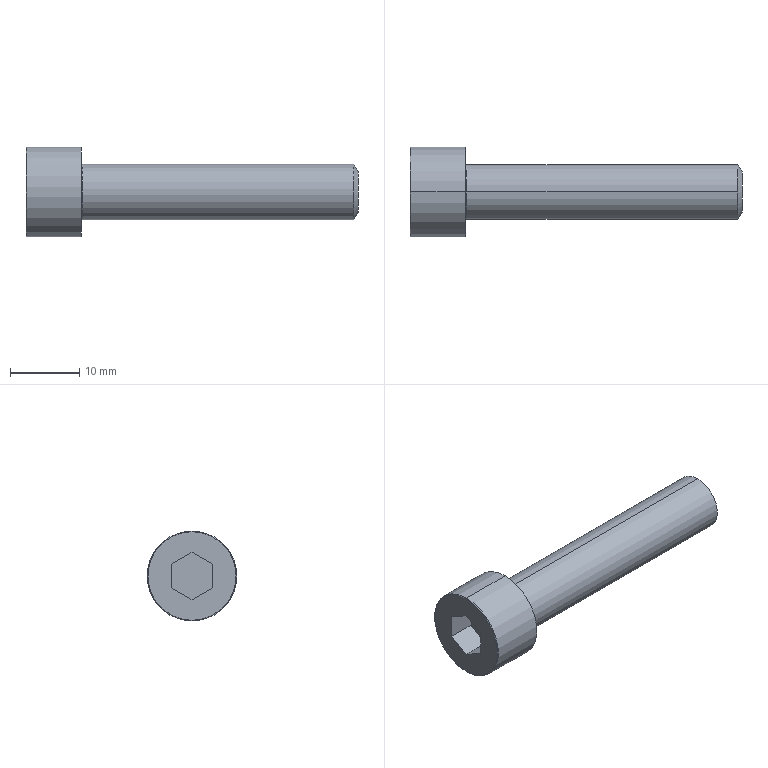Part | SolidWorks | features BlendCut 1, Cut 1, Fillet 1, LPattern 1, RevCut 1, Revolution 1 | 1 solid | 20 faces | box 48 x 13 x 13 mm | volume 2943 mm3 | plane 10 | torus 4 | cylinder 4 | cone 2 | commonest cylinder face diameters 8 x2 13 x2
STEP:
#1=CARTESIAN_POINT('',(0.,0.,6.4));
#2=VERTEX_POINT('',#1);
#3=CARTESIAN_POINT('',(0.,0.,-6.4));
#4=VERTEX_POINT('',#3);
#5=CARTESIAN_POINT('',(0.,0.,0.));
#6=DIRECTION('',(-1.,0.,0.));
#7=DIRECTION('',(0.,0.,-1.));
#8=AXIS2_PLACEMENT_3D('',#5,#6,#7);
#9=CIRCLE('',#8,6.4);
#10=EDGE_CURVE('',#2,#4,#9,.T.);
#11=ORIENTED_EDGE('',*,*,#10,.F.);
#12=CARTESIAN_POINT('',(0.1,0.,6.5));
#13=VERTEX_POINT('',#12);
#14=CARTESIAN_POINT('',(0.1,0.,6.4));
#15=DIRECTION('',(0.,1.,0.));
#16=DIRECTION('',(0.,0.,1.));
#17=AXIS2_PLACEMENT_3D('',#14,#15,#16);
#18=CIRCLE('',#17,0.1);
#19=EDGE_CURVE('',#2,#13,#18,.T.);
#20=ORIENTED_EDGE('',*,*,#19,.T.);
#21=CARTESIAN_POINT('',(0.1,0.,-6.5));
#22=VERTEX_POINT('',#21);
#23=CARTESIAN_POINT('',(0.1,0.,0.));
#24=DIRECTION('',(1.,0.,0.));
#25=DIRECTION('',(0.,0.,-1.));
#26=AXIS2_PLACEMENT_3D('',#23,#24,#25);
#27=CIRCLE('',#26,6.5);
#28=EDGE_CURVE('',#22,#13,#27,.T.);
#29=ORIENTED_EDGE('',*,*,#28,.F.);
#30=CARTESIAN_POINT('',(0.1,0.,-6.4));
#31=DIRECTION('',(0.,-1.,0.));
#32=DIRECTION('',(0.,0.,-1.));
#33=AXIS2_PLACEMENT_3D('',#30,#31,#32);
#34=CIRCLE('',#33,0.1);
#35=EDGE_CURVE('',#4,#22,#34,.T.);
#36=ORIENTED_EDGE('',*,*,#35,.F.);
#37=EDGE_LOOP('',(#11,#20,#29,#36));
#38=FACE_OUTER_BOUND('',#37,.T.);
#39=CARTESIAN_POINT('',(0.1,0.,0.));
#40=DIRECTION('',(1.,0.,0.));
#41=DIRECTION('',(0.,0.,-1.));
#42=AXIS2_PLACEMENT_3D('',#39,#40,#41);
#43=TOROIDAL_SURFACE('',#42,6.4,0.1);
#44=ADVANCED_FACE('',(#38),#43,.T.);
#45=CARTESIAN_POINT('',(48.,0.,2.917));
#46=VERTEX_POINT('',#45);
#47=CARTESIAN_POINT('',(48.,0.,-2.917));
#48=VERTEX_POINT('',#47);
#49=CARTESIAN_POINT('',(48.,0.,0.));
#50=DIRECTION('',(-1.,0.,0.));
#51=DIRECTION('',(0.,0.,1.));
#52=AXIS2_PLACEMENT_3D('',#49,#50,#51);
#53=CIRCLE('',#52,2.917);
#54=EDGE_CURVE('',#46,#48,#53,.T.);
#55=ORIENTED_EDGE('',*,*,#54,.T.);
#56=CARTESIAN_POINT('',(47.375,0.,-4.));
#57=VERTEX_POINT('',#56);
#58=CARTESIAN_POINT('',(47.375,0.,-4.));
#59=DIRECTION('',(-0.5,0.,-0.866));
#60=VECTOR('',#59,1000.);
#61=LINE('',#58,#60);
#62=EDGE_CURVE('',#48,#57,#61,.T.);
#63=ORIENTED_EDGE('',*,*,#62,.T.);
#64=CARTESIAN_POINT('',(47.375,0.,4.));
#65=VERTEX_POINT('',#64);
#66=CARTESIAN_POINT('',(47.375,0.,0.));
#67=DIRECTION('',(-1.,0.,0.));
#68=DIRECTION('',(0.,0.,1.));
#69=AXIS2_PLACEMENT_3D('',#66,#67,#68);
#70=CIRCLE('',#69,4.);
#71=EDGE_CURVE('',#65,#57,#70,.T.);
#72=ORIENTED_EDGE('',*,*,#71,.F.);
#73=CARTESIAN_POINT('',(47.375,0.,4.));
#74=DIRECTION('',(-0.5,0.,0.866));
#75=VECTOR('',#74,1000.);
#76=LINE('',#73,#75);
#77=EDGE_CURVE('',#46,#65,#76,.T.);
#78=ORIENTED_EDGE('',*,*,#77,.F.);
#79=EDGE_LOOP('',(#55,#63,#72,#78));
#80=FACE_OUTER_BOUND('',#79,.T.);
#81=CARTESIAN_POINT('',(47.375,0.,0.));
#82=DIRECTION('',(-1.,0.,0.));
#83=DIRECTION('',(0.,0.,1.));
#84=AXIS2_PLACEMENT_3D('',#81,#82,#83);
#85=CONICAL_SURFACE('',#84,4.,1.047);
#86=ADVANCED_FACE('',(#80),#85,.T.);
#87=CARTESIAN_POINT('',(8.,0.,-4.2));
#88=VERTEX_POINT('',#87);
#89=CARTESIAN_POINT('',(8.,0.,4.2));
#90=VERTEX_POINT('',#89);
#91=CARTESIAN_POINT('',(8.,0.,0.));
#92=DIRECTION('',(-1.,0.,0.));
#93=DIRECTION('',(0.,0.,1.));
#94=AXIS2_PLACEMENT_3D('',#91,#92,#93);
#95=CIRCLE('',#94,4.2);
#96=EDGE_CURVE('',#88,#90,#95,.T.);
#97=ORIENTED_EDGE('',*,*,#96,.F.);
#98=CARTESIAN_POINT('',(8.2,0.,-4.));
#99=VERTEX_POINT('',#98);
#100=CARTESIAN_POINT('',(8.2,0.,-4.2));
#101=DIRECTION('',(0.,1.,0.));
#102=DIRECTION('',(0.,0.,1.));
#103=AXIS2_PLACEMENT_3D('',#100,#101,#102);
#104=CIRCLE('',#103,0.2);
#105=EDGE_CURVE('',#88,#99,#104,.T.);
#106=ORIENTED_EDGE('',*,*,#105,.T.);
#107=CARTESIAN_POINT('',(8.2,0.,4.));
#108=VERTEX_POINT('',#107);
#109=CARTESIAN_POINT('',(8.2,0.,0.));
#110=DIRECTION('',(-1.,0.,0.));
#111=DIRECTION('',(0.,0.,1.));
#112=AXIS2_PLACEMENT_3D('',#109,#110,#111);
#113=CIRCLE('',#112,4.);
#114=EDGE_CURVE('',#99,#108,#113,.T.);
#115=ORIENTED_EDGE('',*,*,#114,.T.);
#116=CARTESIAN_POINT('',(8.2,0.,4.2));
#117=DIRECTION('',(0.,-1.,0.));
#118=DIRECTION('',(0.,0.,-1.));
#119=AXIS2_PLACEMENT_3D('',#116,#117,#118);
#120=CIRCLE('',#119,0.2);
#121=EDGE_CURVE('',#90,#108,#120,.T.);
#122=ORIENTED_EDGE('',*,*,#121,.F.);
#123=EDGE_LOOP('',(#97,#106,#115,#122));
#124=FACE_OUTER_BOUND('',#123,.T.);
#125=CARTESIAN_POINT('',(8.2,0.,0.));
#126=DIRECTION('',(-1.,0.,0.));
#127=DIRECTION('',(0.,0.,1.));
#128=AXIS2_PLACEMENT_3D('',#125,#126,#127);
#129=TOROIDAL_SURFACE('',#128,4.2,0.2);
#130=ADVANCED_FACE('',(#124),#129,.F.);
#131=CARTESIAN_POINT('',(8.,0.,6.5));
#132=VERTEX_POINT('',#131);
#133=CARTESIAN_POINT('',(8.,0.,-6.5));
#134=VERTEX_POINT('',#133);
#135=CARTESIAN_POINT('',(8.,0.,0.));
#136=DIRECTION('',(-1.,0.,0.));
#137=DIRECTION('',(0.,0.,1.));
#138=AXIS2_PLACEMENT_3D('',#135,#136,#137);
#139=CIRCLE('',#138,6.5);
#140=EDGE_CURVE('',#132,#134,#139,.T.);
#141=ORIENTED_EDGE('',*,*,#140,.T.);
#142=CARTESIAN_POINT('',(0.,0.,-6.5));
#143=DIRECTION('',(-1.,0.,0.));
#144=VECTOR('',#143,1000.);
#145=LINE('',#142,#144);
#146=EDGE_CURVE('',#134,#22,#145,.T.);
#147=ORIENTED_EDGE('',*,*,#146,.T.);
#148=ORIENTED_EDGE('',*,*,#28,.T.);
#149=CARTESIAN_POINT('',(0.,0.,6.5));
#150=DIRECTION('',(-1.,0.,0.));
#151=VECTOR('',#150,1000.);
#152=LINE('',#149,#151);
#153=EDGE_CURVE('',#132,#13,#152,.T.);
#154=ORIENTED_EDGE('',*,*,#153,.F.);
#155=EDGE_LOOP('',(#141,#147,#148,#154));
#156=FACE_OUTER_BOUND('',#155,.T.);
#157=CARTESIAN_POINT('',(0.,0.,0.));
#158=DIRECTION('',(-1.,0.,0.));
#159=DIRECTION('',(0.,0.,1.));
#160=AXIS2_PLACEMENT_3D('',#157,#158,#159);
#161=CYLINDRICAL_SURFACE('',#160,6.5);
#162=ADVANCED_FACE('',(#156),#161,.T.);
#163=ORIENTED_EDGE('',*,*,#71,.T.);
#164=CARTESIAN_POINT('',(0.,0.,-4.));
#165=DIRECTION('',(-1.,0.,0.));
#166=VECTOR('',#165,1000.);
#167=LINE('',#164,#166);
#168=EDGE_CURVE('',#57,#99,#167,.T.);
#169=ORIENTED_EDGE('',*,*,#168,.T.);
#170=CARTESIAN_POINT('',(8.2,0.,0.));
#171=DIRECTION('',(-1.,0.,0.));
#172=DIRECTION('',(0.,0.,1.));
#173=AXIS2_PLACEMENT_3D('',#170,#171,#172);
#174=CIRCLE('',#173,4.);
#175=EDGE_CURVE('',#108,#99,#174,.T.);
#176=ORIENTED_EDGE('',*,*,#175,.F.);
#177=CARTESIAN_POINT('',(0.,0.,4.));
#178=DIRECTION('',(-1.,0.,0.));
#179=VECTOR('',#178,1000.);
#180=LINE('',#177,#179);
#181=EDGE_CURVE('',#65,#108,#180,.T.);
#182=ORIENTED_EDGE('',*,*,#181,.F.);
#183=EDGE_LOOP('',(#163,#169,#176,#182));
#184=FACE_OUTER_BOUND('',#183,.T.);
#185=CARTESIAN_POINT('',(0.,0.,0.));
#186=DIRECTION('',(-1.,0.,0.));
#187=DIRECTION('',(0.,0.,1.));
#188=AXIS2_PLACEMENT_3D('',#185,#186,#187);
#189=CYLINDRICAL_SURFACE('',#188,4.);
#190=ADVANCED_FACE('',(#184),#189,.T.);
#191=ORIENTED_EDGE('',*,*,#168,.F.);
#192=CARTESIAN_POINT('',(47.375,0.,0.));
#193=DIRECTION('',(-1.,0.,0.));
#194=DIRECTION('',(0.,0.,1.));
#195=AXIS2_PLACEMENT_3D('',#192,#193,#194);
#196=CIRCLE('',#195,4.);
#197=EDGE_CURVE('',#57,#65,#196,.T.);
#198=ORIENTED_EDGE('',*,*,#197,.T.);
#199=ORIENTED_EDGE('',*,*,#181,.T.);
#200=ORIENTED_EDGE('',*,*,#114,.F.);
#201=EDGE_LOOP('',(#191,#198,#199,#200));
#202=FACE_OUTER_BOUND('',#201,.T.);
#203=CARTESIAN_POINT('',(0.,0.,0.));
#204=DIRECTION('',(-1.,0.,0.));
#205=DIRECTION('',(0.,0.,1.));
#206=AXIS2_PLACEMENT_3D('',#203,#204,#205);
#207=CYLINDRICAL_SURFACE('',#206,4.);
#208=ADVANCED_FACE('',(#202),#207,.T.);
#209=CARTESIAN_POINT('',(0.,0.,0.));
#210=DIRECTION('',(-1.,0.,0.));
#211=DIRECTION('',(0.,0.,-1.));
#212=AXIS2_PLACEMENT_3D('',#209,#210,#211);
#213=CIRCLE('',#212,6.4);
#214=EDGE_CURVE('',#4,#2,#213,.T.);
#215=ORIENTED_EDGE('',*,*,#214,.T.);
#216=ORIENTED_EDGE('',*,*,#10,.T.);
#217=EDGE_LOOP('',(#215,#216));
#218=FACE_OUTER_BOUND('',#217,.T.);
#219=CARTESIAN_POINT('',(0.,0.,3.43));
#220=VERTEX_POINT('',#219);
#221=CARTESIAN_POINT('',(0.,2.97,1.715));
#222=VERTEX_POINT('',#221);
#223=CARTESIAN_POINT('',(0.,0.,3.43));
#224=DIRECTION('',(0.,0.866,-0.5));
#225=VECTOR('',#224,1000.);
#226=LINE('',#223,#225);
#227=EDGE_CURVE('',#220,#222,#226,.T.);
#228=ORIENTED_EDGE('',*,*,#227,.F.);
#229=CARTESIAN_POINT('',(0.,-2.97,1.715));
#230=VERTEX_POINT('',#229);
#231=CARTESIAN_POINT('',(0.,-2.97,1.715));
#232=DIRECTION('',(0.,0.866,0.5));
#233=VECTOR('',#232,1000.);
#234=LINE('',#231,#233);
#235=EDGE_CURVE('',#230,#220,#234,.T.);
#236=ORIENTED_EDGE('',*,*,#235,.F.);
#237=CARTESIAN_POINT('',(0.,-2.97,-1.715));
#238=VERTEX_POINT('',#237);
#239=CARTESIAN_POINT('',(0.,-2.97,-1.715));
#240=DIRECTION('',(0.,0.,1.));
#241=VECTOR('',#240,1000.);
#242=LINE('',#239,#241);
#243=EDGE_CURVE('',#238,#230,#242,.T.);
#244=ORIENTED_EDGE('',*,*,#243,.F.);
#245=CARTESIAN_POINT('',(0.,0.,-3.43));
#246=VERTEX_POINT('',#245);
#247=CARTESIAN_POINT('',(0.,0.,-3.43));
#248=DIRECTION('',(0.,-0.866,0.5));
#249=VECTOR('',#248,1000.);
#250=LINE('',#247,#249);
#251=EDGE_CURVE('',#246,#238,#250,.T.);
#252=ORIENTED_EDGE('',*,*,#251,.F.);
#253=CARTESIAN_POINT('',(0.,2.97,-1.715));
#254=VERTEX_POINT('',#253);
#255=CARTESIAN_POINT('',(0.,2.97,-1.715));
#256=DIRECTION('',(0.,-0.866,-0.5));
#257=VECTOR('',#256,1000.);
#258=LINE('',#255,#257);
#259=EDGE_CURVE('',#254,#246,#258,.T.);
#260=ORIENTED_EDGE('',*,*,#259,.F.);
#261=CARTESIAN_POINT('',(0.,2.97,1.715));
#262=DIRECTION('',(0.,0.,-1.));
#263=VECTOR('',#262,1000.);
#264=LINE('',#261,#263);
#265=EDGE_CURVE('',#222,#254,#264,.T.);
#266=ORIENTED_EDGE('',*,*,#265,.F.);
#267=EDGE_LOOP('',(#228,#236,#244,#252,#260,#266));
#268=FACE_BOUND('',#267,.T.);
#269=CARTESIAN_POINT('',(0.,0.,0.));
#270=DIRECTION('',(1.,0.,0.));
#271=DIRECTION('',(0.,0.,-1.));
#272=AXIS2_PLACEMENT_3D('',#269,#270,#271);
#273=PLANE('',#272);
#274=ADVANCED_FACE('',(#218,#268),#273,.F.);
#275=ORIENTED_EDGE('',*,*,#146,.F.);
#276=CARTESIAN_POINT('',(8.,0.,0.));
#277=DIRECTION('',(-1.,0.,0.));
#278=DIRECTION('',(0.,0.,1.));
#279=AXIS2_PLACEMENT_3D('',#276,#277,#278);
#280=CIRCLE('',#279,6.5);
#281=EDGE_CURVE('',#134,#132,#280,.T.);
#282=ORIENTED_EDGE('',*,*,#281,.T.);
#283=ORIENTED_EDGE('',*,*,#153,.T.);
#284=CARTESIAN_POINT('',(0.1,0.,0.));
#285=DIRECTION('',(1.,0.,0.));
#286=DIRECTION('',(0.,0.,-1.));
#287=AXIS2_PLACEMENT_3D('',#284,#285,#286);
#288=CIRCLE('',#287,6.5);
#289=EDGE_CURVE('',#13,#22,#288,.T.);
#290=ORIENTED_EDGE('',*,*,#289,.T.);
#291=EDGE_LOOP('',(#275,#282,#283,#290));
#292=FACE_OUTER_BOUND('',#291,.T.);
#293=CARTESIAN_POINT('',(0.,0.,0.));
#294=DIRECTION('',(-1.,0.,0.));
#295=DIRECTION('',(0.,0.,1.));
#296=AXIS2_PLACEMENT_3D('',#293,#294,#295);
#297=CYLINDRICAL_SURFACE('',#296,6.5);
#298=ADVANCED_FACE('',(#292),#297,.T.);
#299=ORIENTED_EDGE('',*,*,#140,.F.);
#300=ORIENTED_EDGE('',*,*,#281,.F.);
#301=EDGE_LOOP('',(#299,#300));
#302=FACE_OUTER_BOUND('',#301,.T.);
#303=CARTESIAN_POINT('',(8.,0.,0.));
#304=DIRECTION('',(-1.,0.,0.));
#305=DIRECTION('',(0.,0.,1.));
#306=AXIS2_PLACEMENT_3D('',#303,#304,#305);
#307=CIRCLE('',#306,4.2);
#308=EDGE_CURVE('',#90,#88,#307,.T.);
#309=ORIENTED_EDGE('',*,*,#308,.T.);
#310=ORIENTED_EDGE('',*,*,#96,.T.);
#311=EDGE_LOOP('',(#309,#310));
#312=FACE_BOUND('',#311,.T.);
#313=CARTESIAN_POINT('',(8.,6.5,0.));
#314=DIRECTION('',(-1.,0.,0.));
#315=DIRECTION('',(0.,0.,1.));
#316=AXIS2_PLACEMENT_3D('',#313,#314,#315);
#317=PLANE('',#316);
#318=ADVANCED_FACE('',(#302,#312),#317,.F.);
#319=ORIENTED_EDGE('',*,*,#105,.F.);
#320=ORIENTED_EDGE('',*,*,#308,.F.);
#321=ORIENTED_EDGE('',*,*,#121,.T.);
#322=ORIENTED_EDGE('',*,*,#175,.T.);
#323=EDGE_LOOP('',(#319,#320,#321,#322));
#324=FACE_OUTER_BOUND('',#323,.T.);
#325=CARTESIAN_POINT('',(8.2,0.,0.));
#326=DIRECTION('',(-1.,0.,0.));
#327=DIRECTION('',(0.,0.,1.));
#328=AXIS2_PLACEMENT_3D('',#325,#326,#327);
#329=TOROIDAL_SURFACE('',#328,4.2,0.2);
#330=ADVANCED_FACE('',(#324),#329,.F.);
#331=ORIENTED_EDGE('',*,*,#235,.T.);
#332=CARTESIAN_POINT('',(4.,0.,3.43));
#333=VERTEX_POINT('',#332);
#334=CARTESIAN_POINT('',(4.,0.,3.43));
#335=DIRECTION('',(-1.,0.,0.));
#336=VECTOR('',#335,1000.);
#337=LINE('',#334,#336);
#338=EDGE_CURVE('',#333,#220,#337,.T.);
#339=ORIENTED_EDGE('',*,*,#338,.F.);
#340=CARTESIAN_POINT('',(4.,-2.97,1.715));
#341=VERTEX_POINT('',#340);
#342=CARTESIAN_POINT('',(4.,-2.97,1.715));
#343=DIRECTION('',(0.,0.866,0.5));
#344=VECTOR('',#343,1000.);
#345=LINE('',#342,#344);
#346=EDGE_CURVE('',#341,#333,#345,.T.);
#347=ORIENTED_EDGE('',*,*,#346,.F.);
#348=CARTESIAN_POINT('',(4.,-2.97,1.715));
#349=DIRECTION('',(-1.,0.,0.));
#350=VECTOR('',#349,1000.);
#351=LINE('',#348,#350);
#352=EDGE_CURVE('',#341,#230,#351,.T.);
#353=ORIENTED_EDGE('',*,*,#352,.T.);
#354=EDGE_LOOP('',(#331,#339,#347,#353));
#355=FACE_OUTER_BOUND('',#354,.T.);
#356=CARTESIAN_POINT('',(4.,-2.97,1.715));
#357=DIRECTION('',(0.,-0.5,0.866));
#358=DIRECTION('',(0.,-0.866,-0.5));
#359=AXIS2_PLACEMENT_3D('',#356,#357,#358);
#360=PLANE('',#359);
#361=ADVANCED_FACE('',(#355),#360,.F.);
#362=ORIENTED_EDGE('',*,*,#243,.T.);
#363=ORIENTED_EDGE('',*,*,#352,.F.);
#364=CARTESIAN_POINT('',(4.,-2.97,-1.715));
#365=VERTEX_POINT('',#364);
#366=CARTESIAN_POINT('',(4.,-2.97,-1.715));
#367=DIRECTION('',(0.,0.,1.));
#368=VECTOR('',#367,1000.);
#369=LINE('',#366,#368);
#370=EDGE_CURVE('',#365,#341,#369,.T.);
#371=ORIENTED_EDGE('',*,*,#370,.F.);
#372=CARTESIAN_POINT('',(4.,-2.97,-1.715));
#373=DIRECTION('',(-1.,0.,0.));
#374=VECTOR('',#373,1000.);
#375=LINE('',#372,#374);
#376=EDGE_CURVE('',#365,#238,#375,.T.);
#377=ORIENTED_EDGE('',*,*,#376,.T.);
#378=EDGE_LOOP('',(#362,#363,#371,#377));
#379=FACE_OUTER_BOUND('',#378,.T.);
#380=CARTESIAN_POINT('',(4.,-2.97,-1.715));
#381=DIRECTION('',(0.,-1.,0.));
#382=DIRECTION('',(0.,0.,-1.));
#383=AXIS2_PLACEMENT_3D('',#380,#381,#382);
#384=PLANE('',#383);
#385=ADVANCED_FACE('',(#379),#384,.F.);
#386=ORIENTED_EDGE('',*,*,#251,.T.);
#387=ORIENTED_EDGE('',*,*,#376,.F.);
#388=CARTESIAN_POINT('',(4.,0.,-3.43));
#389=VERTEX_POINT('',#388);
#390=CARTESIAN_POINT('',(4.,0.,-3.43));
#391=DIRECTION('',(0.,-0.866,0.5));
#392=VECTOR('',#391,1000.);
#393=LINE('',#390,#392);
#394=EDGE_CURVE('',#389,#365,#393,.T.);
#395=ORIENTED_EDGE('',*,*,#394,.F.);
#396=CARTESIAN_POINT('',(4.,0.,-3.43));
#397=DIRECTION('',(-1.,0.,0.));
#398=VECTOR('',#397,1000.);
#399=LINE('',#396,#398);
#400=EDGE_CURVE('',#389,#246,#399,.T.);
#401=ORIENTED_EDGE('',*,*,#400,.T.);
#402=EDGE_LOOP('',(#386,#387,#395,#401));
#403=FACE_OUTER_BOUND('',#402,.T.);
#404=CARTESIAN_POINT('',(4.,0.,-3.43));
#405=DIRECTION('',(0.,-0.5,-0.866));
#406=DIRECTION('',(0.,0.866,-0.5));
#407=AXIS2_PLACEMENT_3D('',#404,#405,#406);
#408=PLANE('',#407);
#409=ADVANCED_FACE('',(#403),#408,.F.);
#410=ORIENTED_EDGE('',*,*,#259,.T.);
#411=ORIENTED_EDGE('',*,*,#400,.F.);
#412=CARTESIAN_POINT('',(4.,2.97,-1.715));
#413=VERTEX_POINT('',#412);
#414=CARTESIAN_POINT('',(4.,2.97,-1.715));
#415=DIRECTION('',(0.,-0.866,-0.5));
#416=VECTOR('',#415,1000.);
#417=LINE('',#414,#416);
#418=EDGE_CURVE('',#413,#389,#417,.T.);
#419=ORIENTED_EDGE('',*,*,#418,.F.);
#420=CARTESIAN_POINT('',(4.,2.97,-1.715));
#421=DIRECTION('',(-1.,0.,0.));
#422=VECTOR('',#421,1000.);
#423=LINE('',#420,#422);
#424=EDGE_CURVE('',#413,#254,#423,.T.);
#425=ORIENTED_EDGE('',*,*,#424,.T.);
#426=EDGE_LOOP('',(#410,#411,#419,#425));
#427=FACE_OUTER_BOUND('',#426,.T.);
#428=CARTESIAN_POINT('',(4.,2.97,-1.715));
#429=DIRECTION('',(0.,0.5,-0.866));
#430=DIRECTION('',(0.,0.866,0.5));
#431=AXIS2_PLACEMENT_3D('',#428,#429,#430);
#432=PLANE('',#431);
#433=ADVANCED_FACE('',(#427),#432,.F.);
#434=ORIENTED_EDGE('',*,*,#265,.T.);
#435=ORIENTED_EDGE('',*,*,#424,.F.);
#436=CARTESIAN_POINT('',(4.,2.97,1.715));
#437=VERTEX_POINT('',#436);
#438=CARTESIAN_POINT('',(4.,2.97,1.715));
#439=DIRECTION('',(0.,0.,-1.));
#440=VECTOR('',#439,1000.);
#441=LINE('',#438,#440);
#442=EDGE_CURVE('',#437,#413,#441,.T.);
#443=ORIENTED_EDGE('',*,*,#442,.F.);
#444=CARTESIAN_POINT('',(4.,2.97,1.715));
#445=DIRECTION('',(-1.,0.,0.));
#446=VECTOR('',#445,1000.);
#447=LINE('',#444,#446);
#448=EDGE_CURVE('',#437,#222,#447,.T.);
#449=ORIENTED_EDGE('',*,*,#448,.T.);
#450=EDGE_LOOP('',(#434,#435,#443,#449));
#451=FACE_OUTER_BOUND('',#450,.T.);
#452=CARTESIAN_POINT('',(4.,2.97,1.715));
#453=DIRECTION('',(0.,1.,0.));
#454=DIRECTION('',(0.,0.,1.));
#455=AXIS2_PLACEMENT_3D('',#452,#453,#454);
#456=PLANE('',#455);
#457=ADVANCED_FACE('',(#451),#456,.F.);
#458=ORIENTED_EDGE('',*,*,#227,.T.);
#459=ORIENTED_EDGE('',*,*,#448,.F.);
#460=CARTESIAN_POINT('',(4.,0.,3.43));
#461=DIRECTION('',(0.,0.866,-0.5));
#462=VECTOR('',#461,1000.);
#463=LINE('',#460,#462);
#464=EDGE_CURVE('',#333,#437,#463,.T.);
#465=ORIENTED_EDGE('',*,*,#464,.F.);
#466=ORIENTED_EDGE('',*,*,#338,.T.);
#467=EDGE_LOOP('',(#458,#459,#465,#466));
#468=FACE_OUTER_BOUND('',#467,.T.);
#469=CARTESIAN_POINT('',(4.,0.,3.43));
#470=DIRECTION('',(0.,0.5,0.866));
#471=DIRECTION('',(0.,-0.866,0.5));
#472=AXIS2_PLACEMENT_3D('',#469,#470,#471);
#473=PLANE('',#472);
#474=ADVANCED_FACE('',(#468),#473,.F.);
#475=ORIENTED_EDGE('',*,*,#346,.T.);
#476=ORIENTED_EDGE('',*,*,#464,.T.);
#477=ORIENTED_EDGE('',*,*,#442,.T.);
#478=ORIENTED_EDGE('',*,*,#418,.T.);
#479=ORIENTED_EDGE('',*,*,#394,.T.);
#480=ORIENTED_EDGE('',*,*,#370,.T.);
#481=EDGE_LOOP('',(#475,#476,#477,#478,#479,#480));
#482=FACE_OUTER_BOUND('',#481,.T.);
#483=CARTESIAN_POINT('',(4.,-2.97,1.715));
#484=DIRECTION('',(1.,0.,0.));
#485=DIRECTION('',(0.,0.,-1.));
#486=AXIS2_PLACEMENT_3D('',#483,#484,#485);
#487=PLANE('',#486);
#488=ADVANCED_FACE('',(#482),#487,.F.);
#489=ORIENTED_EDGE('',*,*,#62,.F.);
#490=CARTESIAN_POINT('',(48.,0.,0.));
#491=DIRECTION('',(-1.,0.,0.));
#492=DIRECTION('',(0.,0.,1.));
#493=AXIS2_PLACEMENT_3D('',#490,#491,#492);
#494=CIRCLE('',#493,2.917);
#495=EDGE_CURVE('',#48,#46,#494,.T.);
#496=ORIENTED_EDGE('',*,*,#495,.T.);
#497=ORIENTED_EDGE('',*,*,#77,.T.);
#498=ORIENTED_EDGE('',*,*,#197,.F.);
#499=EDGE_LOOP('',(#489,#496,#497,#498));
#500=FACE_OUTER_BOUND('',#499,.T.);
#501=CARTESIAN_POINT('',(47.375,0.,0.));
#502=DIRECTION('',(-1.,0.,0.));
#503=DIRECTION('',(0.,0.,1.));
#504=AXIS2_PLACEMENT_3D('',#501,#502,#503);
#505=CONICAL_SURFACE('',#504,4.,1.047);
#506=ADVANCED_FACE('',(#500),#505,.T.);
#507=ORIENTED_EDGE('',*,*,#54,.F.);
#508=ORIENTED_EDGE('',*,*,#495,.F.);
#509=EDGE_LOOP('',(#507,#508));
#510=FACE_OUTER_BOUND('',#509,.T.);
#511=CARTESIAN_POINT('',(48.,4.,0.));
#512=DIRECTION('',(-1.,0.,0.));
#513=DIRECTION('',(0.,0.,1.));
#514=AXIS2_PLACEMENT_3D('',#511,#512,#513);
#515=PLANE('',#514);
#516=ADVANCED_FACE('',(#510),#515,.F.);
#517=ORIENTED_EDGE('',*,*,#19,.F.);
#518=ORIENTED_EDGE('',*,*,#214,.F.);
#519=ORIENTED_EDGE('',*,*,#35,.T.);
#520=ORIENTED_EDGE('',*,*,#289,.F.);
#521=EDGE_LOOP('',(#517,#518,#519,#520));
#522=FACE_OUTER_BOUND('',#521,.T.);
#523=CARTESIAN_POINT('',(0.1,0.,0.));
#524=DIRECTION('',(1.,0.,0.));
#525=DIRECTION('',(0.,0.,-1.));
#526=AXIS2_PLACEMENT_3D('',#523,#524,#525);
#527=TOROIDAL_SURFACE('',#526,6.4,0.1);
#528=ADVANCED_FACE('',(#522),#527,.T.);
#529=CLOSED_SHELL('',(#44,#86,#130,#162,#190,#208,#274,#298,#318,#330,#361,#385,#409,#433,#457,#474,#488,#506,#516,#528));
#530=MANIFOLD_SOLID_BREP('',#529);
#531=CARTESIAN_POINT('',(0.,0.,0.));
#532=DIRECTION('',(0.,0.,1.));
#533=DIRECTION('',(1.,0.,0.));
#534=AXIS2_PLACEMENT_3D('',#531,#532,#533);
#535=(LENGTH_UNIT()NAMED_UNIT(*)SI_UNIT(.MILLI.,.METRE.));
#536=UNCERTAINTY_MEASURE_WITH_UNIT(LENGTH_MEASURE(0.00001),#535,'','');
#537=(NAMED_UNIT(*)PLANE_ANGLE_UNIT()SI_UNIT($,.RADIAN.));
#538=(NAMED_UNIT(*)SI_UNIT($,.STERADIAN.)SOLID_ANGLE_UNIT());
#539=(GEOMETRIC_REPRESENTATION_CONTEXT(3)GLOBAL_UNCERTAINTY_ASSIGNED_CONTEXT((#536))GLOBAL_UNIT_ASSIGNED_CONTEXT((#535,#537,#538))REPRESENTATION_CONTEXT('',''));
#540=ADVANCED_BREP_SHAPE_REPRESENTATION('',(#530,#534),#539);